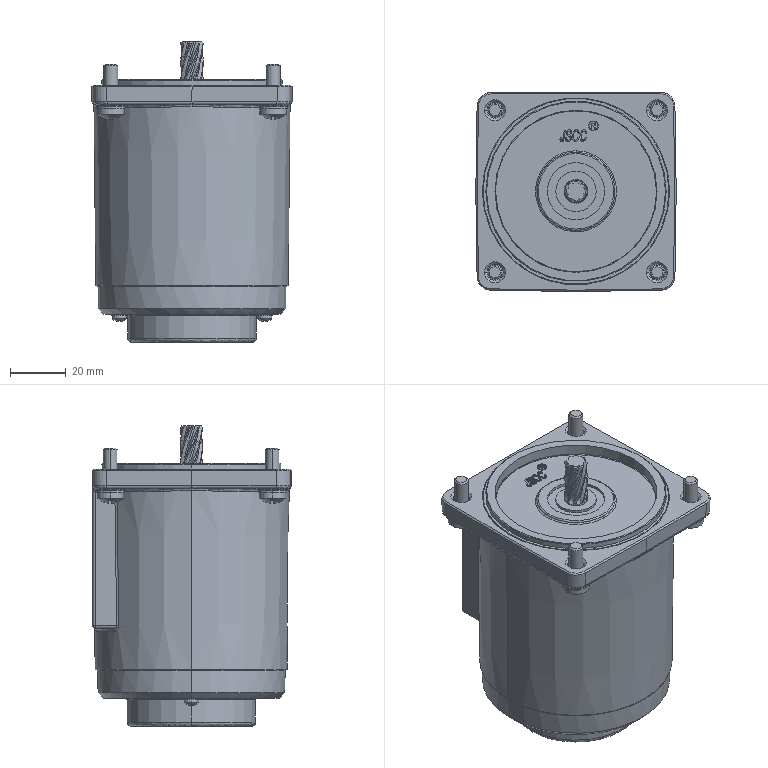Part | STEP file | QA-15YT01-25-1 | 2 solids | 692 faces | box 71.679 x 71.19 x 107.5 mm | volume 89869 mm3 | plane 267 | spline 240 | cylinder 132 | cone 49 | other 4 | commonest cylinder face diameters 1 x16 2 x15 10 x12 3 x8 5 x8 5.8 x8